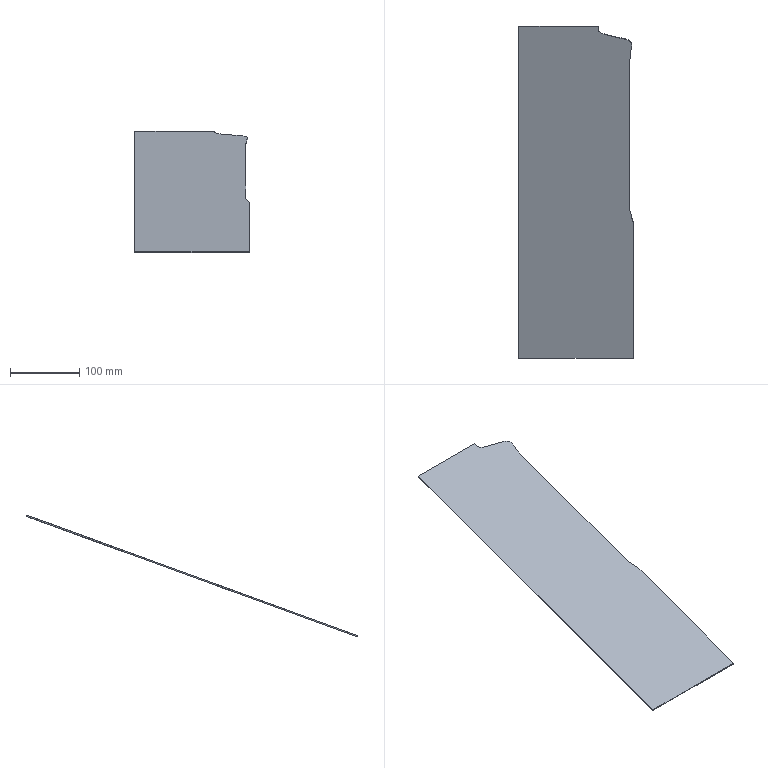Part | NX | features solid 2 | 1 solid | 9 faces | box 165 x 478.472 x 175.78 mm | volume 163563 mm3 | plane 7 | spline 2
STEP:
#1=CARTESIAN_POINT('',(-410.,-162.46,-204.041));
#2=VERTEX_POINT('',#1);
#3=CARTESIAN_POINT('',(-405.,-179.322,-210.178));
#4=VERTEX_POINT('',#3);
#5=CARTESIAN_POINT('',(-405.,-179.322,-210.178));
#6=CARTESIAN_POINT('',(-405.054,-179.151,-210.116));
#7=CARTESIAN_POINT('',(-405.184,-178.753,-209.971));
#8=CARTESIAN_POINT('',(-405.435,-177.992,-209.694));
#9=CARTESIAN_POINT('',(-405.7,-177.191,-209.403));
#10=CARTESIAN_POINT('',(-405.887,-176.625,-209.197));
#11=CARTESIAN_POINT('',(-406.132,-175.87,-208.922));
#12=CARTESIAN_POINT('',(-406.449,-174.871,-208.558));
#13=CARTESIAN_POINT('',(-406.86,-173.48,-208.052));
#14=CARTESIAN_POINT('',(-407.254,-172.054,-207.533));
#15=CARTESIAN_POINT('',(-407.663,-170.503,-206.968));
#16=CARTESIAN_POINT('',(-408.108,-168.795,-206.347));
#17=CARTESIAN_POINT('',(-408.827,-165.935,-205.306));
#18=CARTESIAN_POINT('',(-409.481,-163.808,-204.532));
#19=CARTESIAN_POINT('',(-410.,-162.46,-204.041));
#20=B_SPLINE_CURVE_WITH_KNOTS('',3,(#5,#6,#7,#8,#9,#10,#11,#12,#13,#14,#15,#16,#17,#18,#19),.UNSPECIFIED.,.F.,.F.,(4,1,1,1,1,1,1,1,1,1,1,1,4),(0.,0.0625,0.09375,0.125,0.1562,0.1875,0.25,0.375,0.4375,0.5,0.625,0.75,1.),.UNSPECIFIED.);
#21=EDGE_CURVE('',#2,#4,#20,.F.);
#22=ORIENTED_EDGE('',*,*,#21,.T.);
#23=CARTESIAN_POINT('',(-405.,-178.638,-212.058));
#24=VERTEX_POINT('',#23);
#25=CARTESIAN_POINT('',(-405.,-179.322,-210.178));
#26=CARTESIAN_POINT('',(-405.,-179.094,-210.805));
#27=CARTESIAN_POINT('',(-405.,-178.866,-211.431));
#28=CARTESIAN_POINT('',(-405.,-178.638,-212.058));
#29=B_SPLINE_CURVE_WITH_KNOTS('',3,(#25,#26,#27,#28),.UNSPECIFIED.,.F.,.F.,(4,4),(0.,1.),.UNSPECIFIED.);
#30=EDGE_CURVE('',#24,#4,#29,.F.);
#31=ORIENTED_EDGE('',*,*,#30,.F.);
#32=CARTESIAN_POINT('',(-410.,-161.776,-205.92));
#33=VERTEX_POINT('',#32);
#34=CARTESIAN_POINT('',(-405.,-178.638,-212.058));
#35=CARTESIAN_POINT('',(-405.054,-178.467,-211.996));
#36=CARTESIAN_POINT('',(-405.184,-178.069,-211.85));
#37=CARTESIAN_POINT('',(-405.435,-177.308,-211.574));
#38=CARTESIAN_POINT('',(-405.7,-176.507,-211.282));
#39=CARTESIAN_POINT('',(-405.887,-175.941,-211.076));
#40=CARTESIAN_POINT('',(-406.132,-175.186,-210.801));
#41=CARTESIAN_POINT('',(-406.449,-174.187,-210.438));
#42=CARTESIAN_POINT('',(-406.86,-172.796,-209.931));
#43=CARTESIAN_POINT('',(-407.254,-171.369,-209.412));
#44=CARTESIAN_POINT('',(-407.663,-169.818,-208.848));
#45=CARTESIAN_POINT('',(-408.108,-168.111,-208.226));
#46=CARTESIAN_POINT('',(-408.827,-165.251,-207.185));
#47=CARTESIAN_POINT('',(-409.481,-163.124,-206.411));
#48=CARTESIAN_POINT('',(-410.,-161.776,-205.92));
#49=B_SPLINE_CURVE_WITH_KNOTS('',3,(#34,#35,#36,#37,#38,#39,#40,#41,#42,#43,#44,#45,#46,#47,#48),.UNSPECIFIED.,.F.,.F.,(4,1,1,1,1,1,1,1,1,1,1,1,4),(0.,0.0625,0.09375,0.125,0.1562,0.1875,0.25,0.375,0.4375,0.5,0.625,0.75,1.),.UNSPECIFIED.);
#50=EDGE_CURVE('',#33,#24,#49,.F.);
#51=ORIENTED_EDGE('',*,*,#50,.F.);
#52=CARTESIAN_POINT('',(-410.,-161.776,-205.92));
#53=CARTESIAN_POINT('',(-410.,-162.004,-205.294));
#54=CARTESIAN_POINT('',(-410.,-162.232,-204.668));
#55=CARTESIAN_POINT('',(-410.,-162.46,-204.041));
#56=B_SPLINE_CURVE_WITH_KNOTS('',3,(#52,#53,#54,#55),.UNSPECIFIED.,.F.,.F.,(4,4),(0.,1.),.UNSPECIFIED.);
#57=EDGE_CURVE('',#33,#2,#56,.T.);
#58=ORIENTED_EDGE('',*,*,#57,.T.);
#59=EDGE_LOOP('',(#22,#31,#51,#58));
#60=FACE_BOUND('',#59,.T.);
#61=CARTESIAN_POINT('',(-405.,-178.638,-212.058));
#62=CARTESIAN_POINT('',(-405.,-179.322,-210.178));
#63=CARTESIAN_POINT('',(-405.054,-178.467,-211.996));
#64=CARTESIAN_POINT('',(-405.054,-179.151,-210.116));
#65=CARTESIAN_POINT('',(-405.184,-178.069,-211.85));
#66=CARTESIAN_POINT('',(-405.184,-178.753,-209.971));
#67=CARTESIAN_POINT('',(-405.435,-177.308,-211.574));
#68=CARTESIAN_POINT('',(-405.435,-177.992,-209.694));
#69=CARTESIAN_POINT('',(-405.7,-176.507,-211.282));
#70=CARTESIAN_POINT('',(-405.7,-177.191,-209.403));
#71=CARTESIAN_POINT('',(-405.887,-175.941,-211.076));
#72=CARTESIAN_POINT('',(-405.887,-176.625,-209.197));
#73=CARTESIAN_POINT('',(-406.132,-175.186,-210.801));
#74=CARTESIAN_POINT('',(-406.132,-175.87,-208.922));
#75=CARTESIAN_POINT('',(-406.449,-174.187,-210.438));
#76=CARTESIAN_POINT('',(-406.449,-174.871,-208.558));
#77=CARTESIAN_POINT('',(-406.86,-172.796,-209.931));
#78=CARTESIAN_POINT('',(-406.86,-173.48,-208.052));
#79=CARTESIAN_POINT('',(-407.254,-171.369,-209.412));
#80=CARTESIAN_POINT('',(-407.254,-172.054,-207.533));
#81=CARTESIAN_POINT('',(-407.663,-169.818,-208.848));
#82=CARTESIAN_POINT('',(-407.663,-170.503,-206.968));
#83=CARTESIAN_POINT('',(-408.108,-168.111,-208.226));
#84=CARTESIAN_POINT('',(-408.108,-168.795,-206.347));
#85=CARTESIAN_POINT('',(-408.827,-165.251,-207.185));
#86=CARTESIAN_POINT('',(-408.827,-165.935,-205.306));
#87=CARTESIAN_POINT('',(-409.481,-163.124,-206.411));
#88=CARTESIAN_POINT('',(-409.481,-163.808,-204.532));
#89=CARTESIAN_POINT('',(-410.,-161.776,-205.92));
#90=CARTESIAN_POINT('',(-410.,-162.46,-204.041));
#91=B_SPLINE_SURFACE_WITH_KNOTS('',3,1,((#61,#62),(#63,#64),(#65,#66),(#67,#68),(#69,#70),(#71,#72),(#73,#74),(#75,#76),(#77,#78),(#79,#80),(#81,#82),(#83,#84),(#85,#86),(#87,#88),(#89,#90)),.SURF_OF_LINEAR_EXTRUSION.,.F.,.F.,.F.,(4,1,1,1,1,1,1,1,1,1,1,1,4),(2,2),(0.,0.0625,0.09375,0.125,0.1562,0.1875,0.25,0.375,0.4375,0.5,0.625,0.75,1.),(0.,1.),.UNSPECIFIED.);
#92=ADVANCED_FACE('',(#60),#91,.T.);
#93=CARTESIAN_POINT('',(-410.,53.131,-125.573));
#94=VERTEX_POINT('',#93);
#95=CARTESIAN_POINT('',(-410.,-119.469,-188.394));
#96=DIRECTION('',(0.,-0.9397,-0.342));
#97=VECTOR('',#96,1000.);
#98=LINE('',#95,#97);
#99=EDGE_CURVE('',#94,#2,#98,.T.);
#100=ORIENTED_EDGE('',*,*,#99,.T.);
#101=ORIENTED_EDGE('',*,*,#57,.F.);
#102=CARTESIAN_POINT('',(-410.,53.815,-127.452));
#103=VERTEX_POINT('',#102);
#104=CARTESIAN_POINT('',(-410.,-118.785,-190.273));
#105=DIRECTION('',(0.,-0.9397,-0.342));
#106=VECTOR('',#105,1000.);
#107=LINE('',#104,#106);
#108=EDGE_CURVE('',#103,#33,#107,.T.);
#109=ORIENTED_EDGE('',*,*,#108,.F.);
#110=CARTESIAN_POINT('',(-410.,53.815,-127.452));
#111=DIRECTION('',(0.,-0.342,0.9397));
#112=VECTOR('',#111,1000.);
#113=LINE('',#110,#112);
#114=EDGE_CURVE('',#103,#94,#113,.T.);
#115=ORIENTED_EDGE('',*,*,#114,.T.);
#116=EDGE_LOOP('',(#100,#101,#109,#115));
#117=FACE_BOUND('',#116,.T.);
#118=CARTESIAN_POINT('',(-410.,-118.785,-190.273));
#119=DIRECTION('',(-1.,0.,0.));
#120=DIRECTION('',(0.,0.,1.));
#121=AXIS2_PLACEMENT_3D('',#118,#119,#120);
#122=PLANE('',#121);
#123=ADVANCED_FACE('',(#117),#122,.F.);
#124=CARTESIAN_POINT('',(-454.934,103.135,-107.372));
#125=VERTEX_POINT('',#124);
#126=CARTESIAN_POINT('',(-410.,53.131,-125.573));
#127=CARTESIAN_POINT('',(-409.872,54.833,-124.953));
#128=CARTESIAN_POINT('',(-409.748,58.25,-123.709));
#129=CARTESIAN_POINT('',(-409.381,63.359,-121.85));
#130=CARTESIAN_POINT('',(-408.21,68.4,-120.015));
#131=CARTESIAN_POINT('',(-407.066,72.586,-118.491));
#132=CARTESIAN_POINT('',(-406.885,75.995,-117.251));
#133=CARTESIAN_POINT('',(-407.374,78.548,-116.321));
#134=CARTESIAN_POINT('',(-408.745,80.805,-115.5));
#135=CARTESIAN_POINT('',(-410.825,82.521,-114.875));
#136=CARTESIAN_POINT('',(-413.32,83.61,-114.479));
#137=CARTESIAN_POINT('',(-416.778,84.54,-114.14));
#138=CARTESIAN_POINT('',(-421.253,85.29,-113.867));
#139=CARTESIAN_POINT('',(-426.499,86.58,-113.398));
#140=CARTESIAN_POINT('',(-431.652,88.212,-112.804));
#141=CARTESIAN_POINT('',(-436.862,89.629,-112.288));
#142=CARTESIAN_POINT('',(-442.184,90.614,-111.929));
#143=CARTESIAN_POINT('',(-446.605,91.495,-111.609));
#144=CARTESIAN_POINT('',(-449.977,92.655,-111.187));
#145=CARTESIAN_POINT('',(-452.408,93.866,-110.746));
#146=CARTESIAN_POINT('',(-454.541,95.549,-110.134));
#147=CARTESIAN_POINT('',(-455.7,98.007,-109.239));
#148=CARTESIAN_POINT('',(-455.322,100.609,-108.292));
#149=CARTESIAN_POINT('',(-455.062,102.288,-107.681));
#150=CARTESIAN_POINT('',(-454.934,103.135,-107.372));
#151=B_SPLINE_CURVE_WITH_KNOTS('',3,(#126,#127,#128,#129,#130,#131,#132,#133,#134,#135,#136,#137,#138,#139,#140,#141,#142,#143,#144,#145,#146,#147,#148,#149,#150),.UNSPECIFIED.,.F.,.F.,(4,1,1,1,1,1,1,1,1,1,1,1,1,1,1,1,1,1,1,1,1,1,4),(0.9489,0.9543,0.9597,0.9651,0.9705,0.9732,0.9759,0.9786,0.9813,0.984,0.9867,0.9921,0.9975,1.003,1.008,1.014,1.019,1.022,1.025,1.027,1.03,1.033,1.035),.UNSPECIFIED.);
#152=EDGE_CURVE('',#125,#94,#151,.F.);
#153=ORIENTED_EDGE('',*,*,#152,.T.);
#154=ORIENTED_EDGE('',*,*,#114,.F.);
#155=CARTESIAN_POINT('',(-454.934,103.819,-109.252));
#156=VERTEX_POINT('',#155);
#157=CARTESIAN_POINT('',(-410.,53.815,-127.452));
#158=CARTESIAN_POINT('',(-409.872,55.517,-126.832));
#159=CARTESIAN_POINT('',(-409.748,58.934,-125.589));
#160=CARTESIAN_POINT('',(-409.381,64.043,-123.729));
#161=CARTESIAN_POINT('',(-408.21,69.084,-121.894));
#162=CARTESIAN_POINT('',(-407.066,73.271,-120.371));
#163=CARTESIAN_POINT('',(-406.885,76.679,-119.13));
#164=CARTESIAN_POINT('',(-407.374,79.233,-118.201));
#165=CARTESIAN_POINT('',(-408.745,81.489,-117.379));
#166=CARTESIAN_POINT('',(-410.825,83.205,-116.755));
#167=CARTESIAN_POINT('',(-413.32,84.294,-116.358));
#168=CARTESIAN_POINT('',(-416.778,85.224,-116.02));
#169=CARTESIAN_POINT('',(-421.253,85.974,-115.747));
#170=CARTESIAN_POINT('',(-426.499,87.264,-115.277));
#171=CARTESIAN_POINT('',(-431.652,88.896,-114.683));
#172=CARTESIAN_POINT('',(-436.862,90.313,-114.168));
#173=CARTESIAN_POINT('',(-442.184,91.299,-113.809));
#174=CARTESIAN_POINT('',(-446.605,92.179,-113.488));
#175=CARTESIAN_POINT('',(-449.977,93.339,-113.066));
#176=CARTESIAN_POINT('',(-452.408,94.551,-112.625));
#177=CARTESIAN_POINT('',(-454.541,96.233,-112.013));
#178=CARTESIAN_POINT('',(-455.7,98.691,-111.118));
#179=CARTESIAN_POINT('',(-455.322,101.293,-110.171));
#180=CARTESIAN_POINT('',(-455.062,102.972,-109.56));
#181=CARTESIAN_POINT('',(-454.934,103.819,-109.252));
#182=B_SPLINE_CURVE_WITH_KNOTS('',3,(#157,#158,#159,#160,#161,#162,#163,#164,#165,#166,#167,#168,#169,#170,#171,#172,#173,#174,#175,#176,#177,#178,#179,#180,#181),.UNSPECIFIED.,.F.,.F.,(4,1,1,1,1,1,1,1,1,1,1,1,1,1,1,1,1,1,1,1,1,1,4),(0.9489,0.9543,0.9597,0.9651,0.9705,0.9732,0.9759,0.9786,0.9813,0.984,0.9867,0.9921,0.9975,1.003,1.008,1.014,1.019,1.022,1.025,1.027,1.03,1.033,1.035),.UNSPECIFIED.);
#183=EDGE_CURVE('',#156,#103,#182,.F.);
#184=ORIENTED_EDGE('',*,*,#183,.F.);
#185=CARTESIAN_POINT('',(-454.934,103.819,-109.252));
#186=DIRECTION('',(0.,-0.342,0.9397));
#187=VECTOR('',#186,1000.);
#188=LINE('',#185,#187);
#189=EDGE_CURVE('',#156,#125,#188,.T.);
#190=ORIENTED_EDGE('',*,*,#189,.T.);
#191=EDGE_LOOP('',(#153,#154,#184,#190));
#192=FACE_BOUND('',#191,.T.);
#193=CARTESIAN_POINT('',(-410.,53.815,-127.452));
#194=CARTESIAN_POINT('',(-410.,53.131,-125.573));
#195=CARTESIAN_POINT('',(-409.971,54.195,-127.314));
#196=CARTESIAN_POINT('',(-409.971,53.511,-125.434));
#197=CARTESIAN_POINT('',(-409.934,54.757,-127.109));
#198=CARTESIAN_POINT('',(-409.934,54.073,-125.23));
#199=CARTESIAN_POINT('',(-409.874,55.824,-126.721));
#200=CARTESIAN_POINT('',(-409.874,55.14,-124.841));
#201=CARTESIAN_POINT('',(-409.823,56.812,-126.361));
#202=CARTESIAN_POINT('',(-409.823,56.128,-124.481));
#203=CARTESIAN_POINT('',(-409.768,57.963,-125.942));
#204=CARTESIAN_POINT('',(-409.768,57.279,-124.063));
#205=CARTESIAN_POINT('',(-409.707,59.174,-125.501));
#206=CARTESIAN_POINT('',(-409.707,58.49,-123.622));
#207=CARTESIAN_POINT('',(-409.645,60.193,-125.13));
#208=CARTESIAN_POINT('',(-409.645,59.509,-123.251));
#209=CARTESIAN_POINT('',(-409.608,60.737,-124.932));
#210=CARTESIAN_POINT('',(-409.608,60.053,-123.053));
#211=CARTESIAN_POINT('',(-409.542,61.582,-124.625));
#212=CARTESIAN_POINT('',(-409.542,60.898,-122.745));
#213=CARTESIAN_POINT('',(-409.44,62.608,-124.251));
#214=CARTESIAN_POINT('',(-409.44,61.924,-122.372));
#215=CARTESIAN_POINT('',(-409.298,63.727,-123.844));
#216=CARTESIAN_POINT('',(-409.298,63.043,-121.965));
#217=CARTESIAN_POINT('',(-409.119,64.849,-123.436));
#218=CARTESIAN_POINT('',(-409.119,64.165,-121.556));
#219=CARTESIAN_POINT('',(-408.936,65.824,-123.081));
#220=CARTESIAN_POINT('',(-408.936,65.14,-121.201));
#221=CARTESIAN_POINT('',(-408.787,66.533,-122.823));
#222=CARTESIAN_POINT('',(-408.787,65.849,-120.943));
#223=CARTESIAN_POINT('',(-408.714,66.867,-122.701));
#224=CARTESIAN_POINT('',(-408.714,66.183,-120.822));
#225=CARTESIAN_POINT('',(-408.662,67.097,-122.617));
#226=CARTESIAN_POINT('',(-408.662,66.413,-120.738));
#227=CARTESIAN_POINT('',(-408.642,67.185,-122.585));
#228=CARTESIAN_POINT('',(-408.642,66.501,-120.706));
#229=CARTESIAN_POINT('',(-408.627,67.246,-122.563));
#230=CARTESIAN_POINT('',(-408.627,66.562,-120.684));
#231=CARTESIAN_POINT('',(-408.577,67.457,-122.487));
#232=CARTESIAN_POINT('',(-408.577,66.773,-120.607));
#233=CARTESIAN_POINT('',(-408.452,67.969,-122.3));
#234=CARTESIAN_POINT('',(-408.452,67.285,-120.421));
#235=CARTESIAN_POINT('',(-408.23,68.865,-121.974));
#236=CARTESIAN_POINT('',(-408.23,68.181,-120.094));
#237=CARTESIAN_POINT('',(-407.89,70.231,-121.477));
#238=CARTESIAN_POINT('',(-407.89,69.547,-119.597));
#239=CARTESIAN_POINT('',(-407.679,71.082,-121.167));
#240=CARTESIAN_POINT('',(-407.679,70.398,-119.288));
#241=CARTESIAN_POINT('',(-407.505,71.834,-120.893));
#242=CARTESIAN_POINT('',(-407.505,71.15,-119.014));
#243=CARTESIAN_POINT('',(-407.354,72.533,-120.639));
#244=CARTESIAN_POINT('',(-407.354,71.848,-118.76));
#245=CARTESIAN_POINT('',(-407.232,73.151,-120.414));
#246=CARTESIAN_POINT('',(-407.232,72.467,-118.534));
#247=CARTESIAN_POINT('',(-407.146,73.669,-120.225));
#248=CARTESIAN_POINT('',(-407.146,72.985,-118.346));
#249=CARTESIAN_POINT('',(-407.104,73.953,-120.122));
#250=CARTESIAN_POINT('',(-407.104,73.269,-118.243));
#251=CARTESIAN_POINT('',(-407.022,74.62,-119.879));
#252=CARTESIAN_POINT('',(-407.022,73.936,-118.));
#253=CARTESIAN_POINT('',(-406.948,75.582,-119.529));
#254=CARTESIAN_POINT('',(-406.948,74.898,-117.65));
#255=CARTESIAN_POINT('',(-406.981,77.027,-119.003));
#256=CARTESIAN_POINT('',(-406.981,76.343,-117.124));
#257=CARTESIAN_POINT('',(-407.182,78.262,-118.554));
#258=CARTESIAN_POINT('',(-407.182,77.578,-116.675));
#259=CARTESIAN_POINT('',(-407.66,79.581,-118.074));
#260=CARTESIAN_POINT('',(-407.66,78.897,-116.194));
#261=CARTESIAN_POINT('',(-408.307,80.768,-117.642));
#262=CARTESIAN_POINT('',(-408.307,80.084,-115.762));
#263=CARTESIAN_POINT('',(-409.171,81.813,-117.261));
#264=CARTESIAN_POINT('',(-409.171,81.129,-115.382));
#265=CARTESIAN_POINT('',(-410.308,82.731,-116.927));
#266=CARTESIAN_POINT('',(-410.308,82.047,-115.048));
#267=CARTESIAN_POINT('',(-411.219,83.317,-116.714));
#268=CARTESIAN_POINT('',(-411.219,82.633,-114.834));
#269=CARTESIAN_POINT('',(-412.233,83.817,-116.532));
#270=CARTESIAN_POINT('',(-412.233,83.133,-114.652));
#271=CARTESIAN_POINT('',(-413.345,84.239,-116.378));
#272=CARTESIAN_POINT('',(-413.345,83.555,-114.499));
#273=CARTESIAN_POINT('',(-414.047,84.468,-116.295));
#274=CARTESIAN_POINT('',(-414.047,83.784,-114.416));
#275=CARTESIAN_POINT('',(-414.713,84.658,-116.226));
#276=CARTESIAN_POINT('',(-414.713,83.974,-114.346));
#277=CARTESIAN_POINT('',(-415.037,84.745,-116.194));
#278=CARTESIAN_POINT('',(-415.037,84.061,-114.315));
#279=CARTESIAN_POINT('',(-415.813,84.943,-116.122));
#280=CARTESIAN_POINT('',(-415.813,84.259,-114.243));
#281=CARTESIAN_POINT('',(-416.722,85.148,-116.047));
#282=CARTESIAN_POINT('',(-416.722,84.464,-114.168));
#283=CARTESIAN_POINT('',(-417.651,85.341,-115.977));
#284=CARTESIAN_POINT('',(-417.651,84.657,-114.098));
#285=CARTESIAN_POINT('',(-418.182,85.446,-115.939));
#286=CARTESIAN_POINT('',(-418.182,84.762,-114.059));
#287=CARTESIAN_POINT('',(-418.824,85.57,-115.894));
#288=CARTESIAN_POINT('',(-418.824,84.886,-114.014));
#289=CARTESIAN_POINT('',(-419.702,85.74,-115.832));
#290=CARTESIAN_POINT('',(-419.702,85.056,-113.953));
#291=CARTESIAN_POINT('',(-420.787,85.951,-115.755));
#292=CARTESIAN_POINT('',(-420.787,85.267,-113.876));
#293=CARTESIAN_POINT('',(-421.456,86.083,-115.707));
#294=CARTESIAN_POINT('',(-421.456,85.399,-113.828));
#295=CARTESIAN_POINT('',(-421.831,86.159,-115.68));
#296=CARTESIAN_POINT('',(-421.831,85.475,-113.8));
#297=CARTESIAN_POINT('',(-421.91,86.175,-115.674));
#298=CARTESIAN_POINT('',(-421.91,85.491,-113.794));
#299=CARTESIAN_POINT('',(-422.036,86.201,-115.664));
#300=CARTESIAN_POINT('',(-422.036,85.517,-113.785));
#301=CARTESIAN_POINT('',(-422.264,86.25,-115.646));
#302=CARTESIAN_POINT('',(-422.264,85.566,-113.767));
#303=CARTESIAN_POINT('',(-422.616,86.326,-115.619));
#304=CARTESIAN_POINT('',(-422.616,85.642,-113.739));
#305=CARTESIAN_POINT('',(-423.145,86.446,-115.575));
#306=CARTESIAN_POINT('',(-423.145,85.762,-113.696));
#307=CARTESIAN_POINT('',(-423.984,86.646,-115.502));
#308=CARTESIAN_POINT('',(-423.984,85.962,-113.623));
#309=CARTESIAN_POINT('',(-424.709,86.83,-115.435));
#310=CARTESIAN_POINT('',(-424.709,86.146,-113.556));
#311=CARTESIAN_POINT('',(-425.366,87.008,-115.371));
#312=CARTESIAN_POINT('',(-425.366,86.324,-113.491));
#313=CARTESIAN_POINT('',(-425.664,87.089,-115.341));
#314=CARTESIAN_POINT('',(-425.664,86.405,-113.461));
#315=CARTESIAN_POINT('',(-426.317,87.272,-115.274));
#316=CARTESIAN_POINT('',(-426.317,86.588,-113.395));
#317=CARTESIAN_POINT('',(-427.147,87.512,-115.187));
#318=CARTESIAN_POINT('',(-427.147,86.828,-113.308));
#319=CARTESIAN_POINT('',(-428.008,87.767,-115.094));
#320=CARTESIAN_POINT('',(-428.008,87.083,-113.215));
#321=CARTESIAN_POINT('',(-428.502,87.914,-115.041));
#322=CARTESIAN_POINT('',(-428.502,87.23,-113.161));
#323=CARTESIAN_POINT('',(-429.119,88.1,-114.973));
#324=CARTESIAN_POINT('',(-429.119,87.416,-113.094));
#325=CARTESIAN_POINT('',(-429.947,88.348,-114.883));
#326=CARTESIAN_POINT('',(-429.947,87.664,-113.003));
#327=CARTESIAN_POINT('',(-430.994,88.662,-114.769));
#328=CARTESIAN_POINT('',(-430.994,87.978,-112.889));
#329=CARTESIAN_POINT('',(-431.655,88.858,-114.697));
#330=CARTESIAN_POINT('',(-431.655,88.174,-112.818));
#331=CARTESIAN_POINT('',(-432.073,88.982,-114.652));
#332=CARTESIAN_POINT('',(-432.073,88.298,-112.773));
#333=CARTESIAN_POINT('',(-432.22,89.025,-114.636));
#334=CARTESIAN_POINT('',(-432.22,88.341,-112.757));
#335=CARTESIAN_POINT('',(-432.955,89.236,-114.559));
#336=CARTESIAN_POINT('',(-432.955,88.552,-112.68));
#337=CARTESIAN_POINT('',(-433.641,89.427,-114.49));
#338=CARTESIAN_POINT('',(-433.641,88.743,-112.611));
#339=CARTESIAN_POINT('',(-434.575,89.681,-114.398));
#340=CARTESIAN_POINT('',(-434.575,88.997,-112.518));
#341=CARTESIAN_POINT('',(-435.652,89.957,-114.297));
#342=CARTESIAN_POINT('',(-435.652,89.273,-112.418));
#343=CARTESIAN_POINT('',(-436.844,90.237,-114.195));
#344=CARTESIAN_POINT('',(-436.844,89.552,-112.316));
#345=CARTESIAN_POINT('',(-438.216,90.533,-114.087));
#346=CARTESIAN_POINT('',(-438.216,89.849,-112.208));
#347=CARTESIAN_POINT('',(-439.811,90.852,-113.972));
#348=CARTESIAN_POINT('',(-439.811,90.168,-112.092));
#349=CARTESIAN_POINT('',(-441.092,91.1,-113.881));
#350=CARTESIAN_POINT('',(-441.092,90.416,-112.002));
#351=CARTESIAN_POINT('',(-442.247,91.324,-113.8));
#352=CARTESIAN_POINT('',(-442.247,90.64,-111.92));
#353=CARTESIAN_POINT('',(-443.121,91.489,-113.739));
#354=CARTESIAN_POINT('',(-443.121,90.805,-111.86));
#355=CARTESIAN_POINT('',(-444.633,91.784,-113.632));
#356=CARTESIAN_POINT('',(-444.633,91.1,-111.753));
#357=CARTESIAN_POINT('',(-446.171,92.144,-113.501));
#358=CARTESIAN_POINT('',(-446.171,91.46,-111.622));
#359=CARTESIAN_POINT('',(-447.74,92.591,-113.338));
#360=CARTESIAN_POINT('',(-447.74,91.907,-111.459));
#361=CARTESIAN_POINT('',(-448.609,92.876,-113.235));
#362=CARTESIAN_POINT('',(-448.609,92.191,-111.355));
#363=CARTESIAN_POINT('',(-449.19,93.088,-113.157));
#364=CARTESIAN_POINT('',(-449.19,92.404,-111.278));
#365=CARTESIAN_POINT('',(-449.47,93.196,-113.118));
#366=CARTESIAN_POINT('',(-449.47,92.512,-111.239));
#367=CARTESIAN_POINT('',(-449.881,93.36,-113.059));
#368=CARTESIAN_POINT('',(-449.881,92.676,-111.179));
#369=CARTESIAN_POINT('',(-450.479,93.617,-112.965));
#370=CARTESIAN_POINT('',(-450.479,92.933,-111.086));
#371=CARTESIAN_POINT('',(-451.306,94.013,-112.821));
#372=CARTESIAN_POINT('',(-451.306,93.329,-110.942));
#373=CARTESIAN_POINT('',(-452.241,94.532,-112.632));
#374=CARTESIAN_POINT('',(-452.241,93.848,-110.753));
#375=CARTESIAN_POINT('',(-453.469,95.38,-112.323));
#376=CARTESIAN_POINT('',(-453.469,94.696,-110.444));
#377=CARTESIAN_POINT('',(-454.549,96.454,-111.933));
#378=CARTESIAN_POINT('',(-454.549,95.769,-110.053));
#379=CARTESIAN_POINT('',(-455.265,97.747,-111.462));
#380=CARTESIAN_POINT('',(-455.265,97.063,-109.583));
#381=CARTESIAN_POINT('',(-455.523,98.931,-111.031));
#382=CARTESIAN_POINT('',(-455.523,98.247,-109.151));
#383=CARTESIAN_POINT('',(-455.503,99.98,-110.649));
#384=CARTESIAN_POINT('',(-455.503,99.296,-108.77));
#385=CARTESIAN_POINT('',(-455.435,100.544,-110.444));
#386=CARTESIAN_POINT('',(-455.435,99.86,-108.564));
#387=CARTESIAN_POINT('',(-455.289,101.473,-110.106));
#388=CARTESIAN_POINT('',(-455.289,100.788,-108.226));
#389=CARTESIAN_POINT('',(-455.132,102.517,-109.726));
#390=CARTESIAN_POINT('',(-455.132,101.833,-107.846));
#391=CARTESIAN_POINT('',(-454.999,103.388,-109.409));
#392=CARTESIAN_POINT('',(-454.999,102.704,-107.529));
#393=CARTESIAN_POINT('',(-454.934,103.819,-109.252));
#394=CARTESIAN_POINT('',(-454.934,103.135,-107.372));
#395=B_SPLINE_SURFACE_WITH_KNOTS('',3,1,((#193,#194),(#195,#196),(#197,#198),(#199,#200),(#201,#202),(#203,#204),(#205,#206),(#207,#208),(#209,#210),(#211,#212),(#213,#214),(#215,#216),(#217,#218),(#219,#220),(#221,#222),(#223,#224),(#225,#226),(#227,#228),(#229,#230),(#231,#232),(#233,#234),(#235,#236),(#237,#238),(#239,#240),(#241,#242),(#243,#244),(#245,#246),(#247,#248),(#249,#250),(#251,#252),(#253,#254),(#255,#256),(#257,#258),(#259,#260),(#261,#262),(#263,#264),(#265,#266),(#267,#268),(#269,#270),(#271,#272),(#273,#274),(#275,#276),(#277,#278),(#279,#280),(#281,#282),(#283,#284),(#285,#286),(#287,#288),(#289,#290),(#291,#292),(#293,#294),(#295,#296),(#297,#298),(#299,#300),(#301,#302),(#303,#304),(#305,#306),(#307,#308),(#309,#310),(#311,#312),(#313,#314),(#315,#316),(#317,#318),(#319,#320),(#321,#322),(#323,#324),(#325,#326),(#327,#328),(#329,#330),(#331,#332),(#333,#334),(#335,#336),(#337,#338),(#339,#340),(#341,#342),(#343,#344),(#345,#346),(#347,#348),(#349,#350),(#351,#352),(#353,#354),(#355,#356),(#357,#358),(#359,#360),(#361,#362),(#363,#364),(#365,#366),(#367,#368),(#369,#370),(#371,#372),(#373,#374),(#375,#376),(#377,#378),(#379,#380),(#381,#382),(#383,#384),(#385,#386),(#387,#388),(#389,#390),(#391,#392),(#393,#394)),.SURF_OF_LINEAR_EXTRUSION.,.F.,.F.,.F.,(4,1,1,1,1,1,1,1,1,1,1,1,1,1,1,1,1,1,1,1,1,1,1,1,1,1,1,1,1,1,1,1,1,1,1,1,1,1,1,1,1,1,1,1,1,1,1,1,1,1,1,1,1,1,1,1,1,1,1,1,1,1,1,1,1,1,1,1,1,1,1,1,1,1,1,1,1,1,1,1,1,1,1,1,1,1,1,1,1,1,1,1,1,1,1,1,1,1,4),(2,2),(0.639,0.6449,0.6507,0.6537,0.6566,0.6625,0.6683,0.6713,0.6742,0.6801,0.686,0.6918,0.6977,0.7006,0.7021,0.7028,0.7036,0.705,0.7065,0.7094,0.7153,0.7182,0.7212,0.7241,0.727,0.73,0.7329,0.7344,0.7358,0.7388,0.7446,0.7505,0.7534,0.7564,0.7622,0.7652,0.7681,0.774,0.7769,0.7799,0.7813,0.7828,0.7857,0.7916,0.7945,0.796,0.7975,0.8004,0.8033,0.8092,0.8107,0.8121,0.8129,0.8136,0.8151,0.818,0.8209,0.8268,0.8283,0.8297,0.8327,0.8385,0.8415,0.8429,0.8444,0.8473,0.8503,0.8561,0.8576,0.8591,0.862,0.865,0.8679,0.8738,0.8796,0.8855,0.8914,0.8972,0.9031,0.906,0.909,0.9207,0.9266,0.9324,0.9354,0.9368,0.9383,0.9412,0.9442,0.95,0.9559,0.9677,0.9794,0.9911,0.997,0.9999,1.003,1.009,1.015),(0.,1.),.UNSPECIFIED.);
#396=ADVANCED_FACE('',(#192),#395,.T.);
#397=CARTESIAN_POINT('',(-570.,103.135,-107.372));
#398=VERTEX_POINT('',#397);
#399=CARTESIAN_POINT('',(-640.,103.135,-107.372));
#400=DIRECTION('',(-1.,0.,0.));
#401=VECTOR('',#400,1000.);
#402=LINE('',#399,#401);
#403=EDGE_CURVE('',#125,#398,#402,.T.);
#404=ORIENTED_EDGE('',*,*,#403,.F.);
#405=ORIENTED_EDGE('',*,*,#189,.F.);
#406=CARTESIAN_POINT('',(-570.,103.819,-109.252));
#407=VERTEX_POINT('',#406);
#408=CARTESIAN_POINT('',(-640.,103.819,-109.252));
#409=DIRECTION('',(-1.,0.,0.));
#410=VECTOR('',#409,1000.);
#411=LINE('',#408,#410);
#412=EDGE_CURVE('',#156,#407,#411,.T.);
#413=ORIENTED_EDGE('',*,*,#412,.T.);
#414=CARTESIAN_POINT('',(-570.,103.819,-109.252));
#415=DIRECTION('',(0.,-0.342,0.9397));
#416=VECTOR('',#415,1000.);
#417=LINE('',#414,#416);
#418=EDGE_CURVE('',#407,#398,#417,.T.);
#419=ORIENTED_EDGE('',*,*,#418,.T.);
#420=EDGE_LOOP('',(#404,#405,#413,#419));
#421=FACE_BOUND('',#420,.T.);
#422=CARTESIAN_POINT('',(-459.422,103.819,-109.252));
#423=DIRECTION('',(0.,0.9397,0.342));
#424=DIRECTION('',(0.,-0.342,0.9397));
#425=AXIS2_PLACEMENT_3D('',#422,#423,#424);
#426=PLANE('',#425);
#427=ADVANCED_FACE('',(#421),#426,.T.);
#428=CARTESIAN_POINT('',(-570.,-374.653,-281.273));
#429=VERTEX_POINT('',#428);
#430=CARTESIAN_POINT('',(-570.,-419.123,-297.459));
#431=DIRECTION('',(0.,-0.9397,-0.342));
#432=VECTOR('',#431,1000.);
#433=LINE('',#430,#432);
#434=EDGE_CURVE('',#398,#429,#433,.T.);
#435=ORIENTED_EDGE('',*,*,#434,.F.);
#436=ORIENTED_EDGE('',*,*,#418,.F.);
#437=CARTESIAN_POINT('',(-570.,-373.969,-283.152));
#438=VERTEX_POINT('',#437);
#439=CARTESIAN_POINT('',(-570.,-418.439,-299.338));
#440=DIRECTION('',(0.,-0.9397,-0.342));
#441=VECTOR('',#440,1000.);
#442=LINE('',#439,#441);
#443=EDGE_CURVE('',#407,#438,#442,.T.);
#444=ORIENTED_EDGE('',*,*,#443,.T.);
#445=CARTESIAN_POINT('',(-570.,-373.969,-283.152));
#446=DIRECTION('',(0.,-0.342,0.9397));
#447=VECTOR('',#446,1000.);
#448=LINE('',#445,#447);
#449=EDGE_CURVE('',#438,#429,#448,.T.);
#450=ORIENTED_EDGE('',*,*,#449,.T.);
#451=EDGE_LOOP('',(#435,#436,#444,#450));
#452=FACE_BOUND('',#451,.T.);
#453=CARTESIAN_POINT('',(-570.,-418.439,-299.338));
#454=DIRECTION('',(-1.,0.,0.));
#455=DIRECTION('',(0.,-1.,0.));
#456=AXIS2_PLACEMENT_3D('',#453,#454,#455);
#457=PLANE('',#456);
#458=ADVANCED_FACE('',(#452),#457,.T.);
#459=CARTESIAN_POINT('',(-405.,-374.653,-281.273));
#460=VERTEX_POINT('',#459);
#461=CARTESIAN_POINT('',(-640.,-374.653,-281.273));
#462=DIRECTION('',(-1.,0.,0.));
#463=VECTOR('',#462,1000.);
#464=LINE('',#461,#463);
#465=EDGE_CURVE('',#460,#429,#464,.T.);
#466=ORIENTED_EDGE('',*,*,#465,.T.);
#467=ORIENTED_EDGE('',*,*,#449,.F.);
#468=CARTESIAN_POINT('',(-405.,-373.969,-283.152));
#469=VERTEX_POINT('',#468);
#470=CARTESIAN_POINT('',(-640.,-373.969,-283.152));
#471=DIRECTION('',(-1.,0.,0.));
#472=VECTOR('',#471,1000.);
#473=LINE('',#470,#472);
#474=EDGE_CURVE('',#469,#438,#473,.T.);
#475=ORIENTED_EDGE('',*,*,#474,.F.);
#476=CARTESIAN_POINT('',(-405.,-373.969,-283.152));
#477=DIRECTION('',(0.,-0.342,0.9397));
#478=VECTOR('',#477,1000.);
#479=LINE('',#476,#478);
#480=EDGE_CURVE('',#469,#460,#479,.T.);
#481=ORIENTED_EDGE('',*,*,#480,.T.);
#482=EDGE_LOOP('',(#466,#467,#475,#481));
#483=FACE_BOUND('',#482,.T.);
#484=CARTESIAN_POINT('',(-690.,-373.969,-283.152));
#485=DIRECTION('',(0.,0.9397,0.342));
#486=DIRECTION('',(0.,-0.342,0.9397));
#487=AXIS2_PLACEMENT_3D('',#484,#485,#486);
#488=PLANE('',#487);
#489=ADVANCED_FACE('',(#483),#488,.F.);
#490=CARTESIAN_POINT('',(-405.,102.736,-107.518));
#491=DIRECTION('',(0.,-0.9397,-0.342));
#492=VECTOR('',#491,1000.);
#493=LINE('',#490,#492);
#494=EDGE_CURVE('',#460,#4,#493,.F.);
#495=ORIENTED_EDGE('',*,*,#494,.F.);
#496=ORIENTED_EDGE('',*,*,#480,.F.);
#497=CARTESIAN_POINT('',(-405.,103.42,-109.397));
#498=DIRECTION('',(0.,-0.9397,-0.342));
#499=VECTOR('',#498,1000.);
#500=LINE('',#497,#499);
#501=EDGE_CURVE('',#469,#24,#500,.F.);
#502=ORIENTED_EDGE('',*,*,#501,.T.);
#503=ORIENTED_EDGE('',*,*,#30,.T.);
#504=EDGE_LOOP('',(#495,#496,#502,#503));
#505=FACE_BOUND('',#504,.T.);
#506=CARTESIAN_POINT('',(-405.,103.42,-109.397));
#507=DIRECTION('',(1.,0.,0.));
#508=DIRECTION('',(0.,0.,-1.));
#509=AXIS2_PLACEMENT_3D('',#506,#507,#508);
#510=PLANE('',#509);
#511=ADVANCED_FACE('',(#505),#510,.T.);
#512=ORIENTED_EDGE('',*,*,#50,.T.);
#513=ORIENTED_EDGE('',*,*,#501,.F.);
#514=ORIENTED_EDGE('',*,*,#474,.T.);
#515=ORIENTED_EDGE('',*,*,#443,.F.);
#516=ORIENTED_EDGE('',*,*,#412,.F.);
#517=ORIENTED_EDGE('',*,*,#183,.T.);
#518=ORIENTED_EDGE('',*,*,#108,.T.);
#519=EDGE_LOOP('',(#512,#513,#514,#515,#516,#517,#518));
#520=FACE_BOUND('',#519,.T.);
#521=CARTESIAN_POINT('',(-640.,103.42,-109.397));
#522=DIRECTION('',(0.,-0.342,0.9397));
#523=DIRECTION('',(0.,-0.9397,-0.342));
#524=AXIS2_PLACEMENT_3D('',#521,#522,#523);
#525=PLANE('',#524);
#526=ADVANCED_FACE('',(#520),#525,.F.);
#527=ORIENTED_EDGE('',*,*,#21,.F.);
#528=ORIENTED_EDGE('',*,*,#99,.F.);
#529=ORIENTED_EDGE('',*,*,#152,.F.);
#530=ORIENTED_EDGE('',*,*,#403,.T.);
#531=ORIENTED_EDGE('',*,*,#434,.T.);
#532=ORIENTED_EDGE('',*,*,#465,.F.);
#533=ORIENTED_EDGE('',*,*,#494,.T.);
#534=EDGE_LOOP('',(#527,#528,#529,#530,#531,#532,#533));
#535=FACE_BOUND('',#534,.T.);
#536=CARTESIAN_POINT('',(-640.,102.736,-107.518));
#537=DIRECTION('',(0.,-0.342,0.9397));
#538=DIRECTION('',(0.,-0.9397,-0.342));
#539=AXIS2_PLACEMENT_3D('',#536,#537,#538);
#540=PLANE('',#539);
#541=ADVANCED_FACE('',(#535),#540,.T.);
#542=CLOSED_SHELL('',(#92,#123,#396,#427,#458,#489,#511,#526,#541));
#543=MANIFOLD_SOLID_BREP('',#542);
#544=(LENGTH_UNIT()NAMED_UNIT(*)SI_UNIT(.MILLI.,.METRE.));
#545=UNCERTAINTY_MEASURE_WITH_UNIT(LENGTH_MEASURE(0.0508),#544,'','');
#546=(NAMED_UNIT(*)PLANE_ANGLE_UNIT()SI_UNIT($,.RADIAN.));
#547=(NAMED_UNIT(*)SI_UNIT($,.STERADIAN.)SOLID_ANGLE_UNIT());
#548=(GEOMETRIC_REPRESENTATION_CONTEXT(3)GLOBAL_UNCERTAINTY_ASSIGNED_CONTEXT((#545))GLOBAL_UNIT_ASSIGNED_CONTEXT((#544,#546,#547))REPRESENTATION_CONTEXT('',''));
#549=ADVANCED_BREP_SHAPE_REPRESENTATION('',(#543),#548);